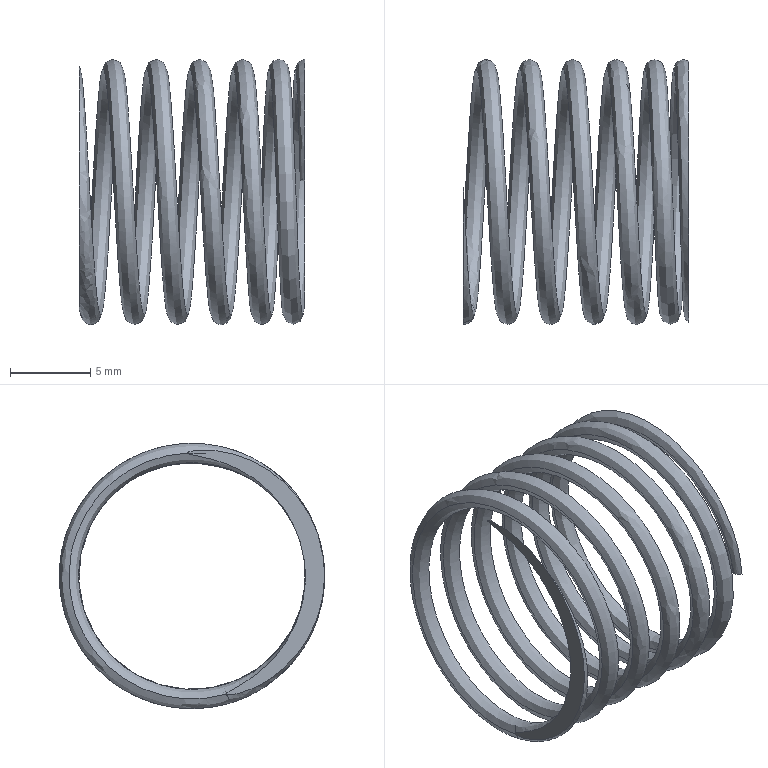Part | NX | features BREP 1 | 1 solid | 5 faces | volume 317.43 mm3 | plane 3 | spline 2